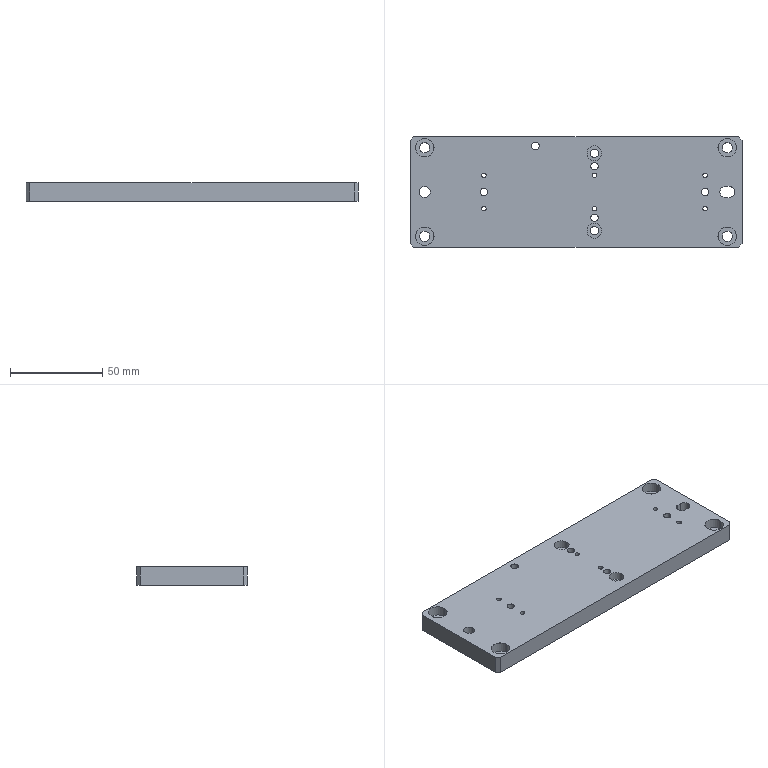Part | STEP file | QA-FB03 | 1 solid | 77 faces | box 180 x 60 x 10 mm | volume 103545 mm3 | cylinder 51 | plane 18 | cone 8 | commonest cylinder face diameters 2.5 x12 4 x8 5.5 x8 10 x8 6 x5 4.5 x4